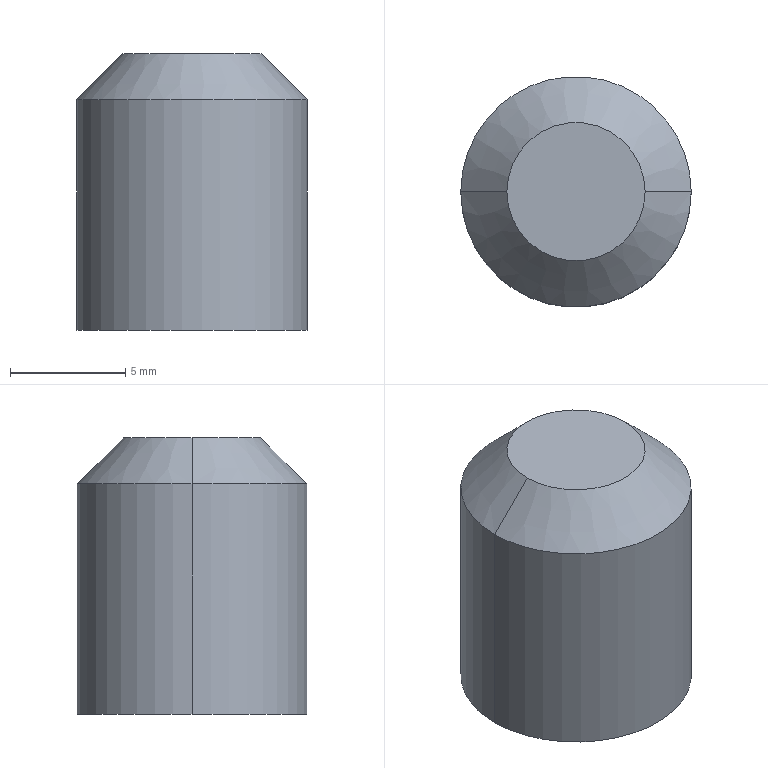Part | STEP file | ASND-0110-Body 1-26 | 1 solid | 6 faces | box 10 x 10 x 12 mm | volume 888.024 mm3 | cylinder 2 | cone 2 | plane 2 | commonest cylinder face diameters 10 x2
STEP:
#1=CARTESIAN_POINT('',(0.,0.,0.));
#2=DIRECTION('',(0.,0.,1.));
#3=DIRECTION('',(1.,0.,0.));
#4=AXIS2_PLACEMENT_3D('',#1,#2,#3);
#5=CARTESIAN_POINT('',(5.,0.,0.));
#6=VERTEX_POINT('',#5);
#7=CARTESIAN_POINT('',(-5.,0.,0.));
#8=VERTEX_POINT('',#7);
#9=CARTESIAN_POINT('',(0.,0.,0.));
#10=DIRECTION('',(0.,0.,-1.));
#11=DIRECTION('',(-1.,0.,0.));
#12=AXIS2_PLACEMENT_3D('',#9,#10,#11);
#13=CIRCLE('',#12,5.);
#14=CARTESIAN_POINT('',(0.,0.,0.));
#15=DIRECTION('',(0.,0.,1.));
#16=DIRECTION('',(-1.,0.,0.));
#17=AXIS2_PLACEMENT_3D('',#14,#15,#16);
#18=CYLINDRICAL_SURFACE('',#17,5.);
#19=CARTESIAN_POINT('',(6.283,0.));
#20=DIRECTION('',(-1.,0.));
#21=VECTOR('',#20,1.);
#22=LINE('',#19,#21);
#23=(GEOMETRIC_REPRESENTATION_CONTEXT(2)PARAMETRIC_REPRESENTATION_CONTEXT()REPRESENTATION_CONTEXT('',''));
#24=DEFINITIONAL_REPRESENTATION('',(#22),#23);
#25=PCURVE('',#18,#24);
#26=CARTESIAN_POINT('',(0.,0.,0.));
#27=DIRECTION('',(0.,0.,-1.));
#28=DIRECTION('',(0.7071,0.7071,0.));
#29=AXIS2_PLACEMENT_3D('',#26,#27,#28);
#30=PLANE('',#29);
#31=CARTESIAN_POINT('',(0.,0.));
#32=DIRECTION('',(-0.7071,-0.7071));
#33=AXIS2_PLACEMENT_2D('',#31,#32);
#34=CIRCLE('',#33,5.);
#35=(GEOMETRIC_REPRESENTATION_CONTEXT(2)PARAMETRIC_REPRESENTATION_CONTEXT()REPRESENTATION_CONTEXT('',''));
#36=DEFINITIONAL_REPRESENTATION('',(#34),#35);
#37=PCURVE('',#30,#36);
#38=SURFACE_CURVE('',#13,(#25,#37),.PCURVE_S1.);
#39=EDGE_CURVE('',#6,#8,#38,.T.);
#40=ORIENTED_EDGE('',*,*,#39,.F.);
#41=CARTESIAN_POINT('',(5.,0.,10.));
#42=VERTEX_POINT('',#41);
#43=CARTESIAN_POINT('',(5.,0.,0.));
#44=DIRECTION('',(0.,0.,1.));
#45=VECTOR('',#44,1.);
#46=LINE('',#43,#45);
#47=CARTESIAN_POINT('',(3.142,0.));
#48=DIRECTION('',(0.,1.));
#49=VECTOR('',#48,1.);
#50=LINE('',#47,#49);
#51=(GEOMETRIC_REPRESENTATION_CONTEXT(2)PARAMETRIC_REPRESENTATION_CONTEXT()REPRESENTATION_CONTEXT('',''));
#52=DEFINITIONAL_REPRESENTATION('',(#50),#51);
#53=PCURVE('',#18,#52);
#54=CARTESIAN_POINT('',(0.,0.,0.));
#55=DIRECTION('',(0.,0.,1.));
#56=DIRECTION('',(-1.,0.,0.));
#57=AXIS2_PLACEMENT_3D('',#54,#55,#56);
#58=CYLINDRICAL_SURFACE('',#57,5.);
#59=CARTESIAN_POINT('',(3.142,0.));
#60=DIRECTION('',(0.,1.));
#61=VECTOR('',#60,1.);
#62=LINE('',#59,#61);
#63=(GEOMETRIC_REPRESENTATION_CONTEXT(2)PARAMETRIC_REPRESENTATION_CONTEXT()REPRESENTATION_CONTEXT('',''));
#64=DEFINITIONAL_REPRESENTATION('',(#62),#63);
#65=PCURVE('',#58,#64);
#66=SURFACE_CURVE('',#46,(#53,#65),.PCURVE_S1.);
#67=EDGE_CURVE('',#6,#42,#66,.T.);
#68=ORIENTED_EDGE('',*,*,#67,.T.);
#69=CARTESIAN_POINT('',(-5.,0.,10.));
#70=VERTEX_POINT('',#69);
#71=CARTESIAN_POINT('',(0.,0.,10.));
#72=DIRECTION('',(0.,0.,1.));
#73=DIRECTION('',(-1.,0.,0.));
#74=AXIS2_PLACEMENT_3D('',#71,#72,#73);
#75=CIRCLE('',#74,5.);
#76=CARTESIAN_POINT('',(0.,10.));
#77=DIRECTION('',(1.,0.));
#78=VECTOR('',#77,1.);
#79=LINE('',#76,#78);
#80=(GEOMETRIC_REPRESENTATION_CONTEXT(2)PARAMETRIC_REPRESENTATION_CONTEXT()REPRESENTATION_CONTEXT('',''));
#81=DEFINITIONAL_REPRESENTATION('',(#79),#80);
#82=PCURVE('',#18,#81);
#83=CARTESIAN_POINT('',(0.,0.,11.));
#84=DIRECTION('',(0.,0.,-1.));
#85=DIRECTION('',(-1.,0.,0.));
#86=AXIS2_PLACEMENT_3D('',#83,#84,#85);
#87=CONICAL_SURFACE('',#86,4.,0.7854);
#88=CARTESIAN_POINT('',(6.283,1.));
#89=DIRECTION('',(-1.,0.));
#90=VECTOR('',#89,1.);
#91=LINE('',#88,#90);
#92=(GEOMETRIC_REPRESENTATION_CONTEXT(2)PARAMETRIC_REPRESENTATION_CONTEXT()REPRESENTATION_CONTEXT('',''));
#93=DEFINITIONAL_REPRESENTATION('',(#91),#92);
#94=PCURVE('',#87,#93);
#95=SURFACE_CURVE('',#75,(#82,#94),.PCURVE_S1.);
#96=EDGE_CURVE('',#70,#42,#95,.T.);
#97=ORIENTED_EDGE('',*,*,#96,.F.);
#98=CARTESIAN_POINT('',(-5.,0.,0.));
#99=DIRECTION('',(0.,0.,1.));
#100=VECTOR('',#99,1.);
#101=LINE('',#98,#100);
#102=CARTESIAN_POINT('',(0.,0.));
#103=DIRECTION('',(0.,1.));
#104=VECTOR('',#103,1.);
#105=LINE('',#102,#104);
#106=(GEOMETRIC_REPRESENTATION_CONTEXT(2)PARAMETRIC_REPRESENTATION_CONTEXT()REPRESENTATION_CONTEXT('',''));
#107=DEFINITIONAL_REPRESENTATION('',(#105),#106);
#108=PCURVE('',#18,#107);
#109=CARTESIAN_POINT('',(6.283,0.));
#110=DIRECTION('',(0.,1.));
#111=VECTOR('',#110,1.);
#112=LINE('',#109,#111);
#113=(GEOMETRIC_REPRESENTATION_CONTEXT(2)PARAMETRIC_REPRESENTATION_CONTEXT()REPRESENTATION_CONTEXT('',''));
#114=DEFINITIONAL_REPRESENTATION('',(#112),#113);
#115=PCURVE('',#58,#114);
#116=SURFACE_CURVE('',#101,(#108,#115),.PCURVE_S1.);
#117=EDGE_CURVE('',#8,#70,#116,.T.);
#118=ORIENTED_EDGE('',*,*,#117,.F.);
#119=EDGE_LOOP('',(#40,#68,#97,#118));
#120=FACE_BOUND('',#119,.T.);
#121=ADVANCED_FACE('',(#120),#18,.T.);
#122=CARTESIAN_POINT('',(-3.,0.,12.));
#123=VERTEX_POINT('',#122);
#124=CARTESIAN_POINT('',(3.,0.,12.));
#125=VERTEX_POINT('',#124);
#126=CARTESIAN_POINT('',(0.,0.,12.));
#127=DIRECTION('',(0.,0.,-1.));
#128=DIRECTION('',(-1.,0.,0.));
#129=AXIS2_PLACEMENT_3D('',#126,#127,#128);
#130=CIRCLE('',#129,3.);
#131=CARTESIAN_POINT('',(0.,0.,11.));
#132=DIRECTION('',(0.,0.,-1.));
#133=DIRECTION('',(-1.,0.,0.));
#134=AXIS2_PLACEMENT_3D('',#131,#132,#133);
#135=CONICAL_SURFACE('',#134,4.,0.7854);
#136=CARTESIAN_POINT('',(0.,-1.));
#137=DIRECTION('',(1.,0.));
#138=VECTOR('',#137,1.);
#139=LINE('',#136,#138);
#140=(GEOMETRIC_REPRESENTATION_CONTEXT(2)PARAMETRIC_REPRESENTATION_CONTEXT()REPRESENTATION_CONTEXT('',''));
#141=DEFINITIONAL_REPRESENTATION('',(#139),#140);
#142=PCURVE('',#135,#141);
#143=CARTESIAN_POINT('',(0.,0.,12.));
#144=DIRECTION('',(0.,0.,-1.));
#145=DIRECTION('',(0.7071,0.7071,0.));
#146=AXIS2_PLACEMENT_3D('',#143,#144,#145);
#147=PLANE('',#146);
#148=CARTESIAN_POINT('',(0.,0.));
#149=DIRECTION('',(-0.7071,-0.7071));
#150=AXIS2_PLACEMENT_2D('',#148,#149);
#151=CIRCLE('',#150,3.);
#152=(GEOMETRIC_REPRESENTATION_CONTEXT(2)PARAMETRIC_REPRESENTATION_CONTEXT()REPRESENTATION_CONTEXT('',''));
#153=DEFINITIONAL_REPRESENTATION('',(#151),#152);
#154=PCURVE('',#147,#153);
#155=SURFACE_CURVE('',#130,(#142,#154),.PCURVE_S1.);
#156=EDGE_CURVE('',#123,#125,#155,.T.);
#157=ORIENTED_EDGE('',*,*,#156,.T.);
#158=CARTESIAN_POINT('',(4.,0.,11.));
#159=DIRECTION('',(0.7071,0.,-0.7071));
#160=VECTOR('',#159,1.);
#161=LINE('',#158,#160);
#162=CARTESIAN_POINT('',(3.142,0.));
#163=DIRECTION('',(0.,1.));
#164=VECTOR('',#163,1.);
#165=LINE('',#162,#164);
#166=(GEOMETRIC_REPRESENTATION_CONTEXT(2)PARAMETRIC_REPRESENTATION_CONTEXT()REPRESENTATION_CONTEXT('',''));
#167=DEFINITIONAL_REPRESENTATION('',(#165),#166);
#168=PCURVE('',#135,#167);
#169=CARTESIAN_POINT('',(3.142,0.));
#170=DIRECTION('',(0.,1.));
#171=VECTOR('',#170,1.);
#172=LINE('',#169,#171);
#173=(GEOMETRIC_REPRESENTATION_CONTEXT(2)PARAMETRIC_REPRESENTATION_CONTEXT()REPRESENTATION_CONTEXT('',''));
#174=DEFINITIONAL_REPRESENTATION('',(#172),#173);
#175=PCURVE('',#87,#174);
#176=SURFACE_CURVE('',#161,(#168,#175),.PCURVE_S1.);
#177=EDGE_CURVE('',#125,#42,#176,.T.);
#178=ORIENTED_EDGE('',*,*,#177,.T.);
#179=CARTESIAN_POINT('',(0.,0.,10.));
#180=DIRECTION('',(0.,0.,1.));
#181=DIRECTION('',(-1.,0.,0.));
#182=AXIS2_PLACEMENT_3D('',#179,#180,#181);
#183=CIRCLE('',#182,5.);
#184=CARTESIAN_POINT('',(6.283,1.));
#185=DIRECTION('',(-1.,0.));
#186=VECTOR('',#185,1.);
#187=LINE('',#184,#186);
#188=(GEOMETRIC_REPRESENTATION_CONTEXT(2)PARAMETRIC_REPRESENTATION_CONTEXT()REPRESENTATION_CONTEXT('',''));
#189=DEFINITIONAL_REPRESENTATION('',(#187),#188);
#190=PCURVE('',#135,#189);
#191=CARTESIAN_POINT('',(0.,10.));
#192=DIRECTION('',(1.,0.));
#193=VECTOR('',#192,1.);
#194=LINE('',#191,#193);
#195=(GEOMETRIC_REPRESENTATION_CONTEXT(2)PARAMETRIC_REPRESENTATION_CONTEXT()REPRESENTATION_CONTEXT('',''));
#196=DEFINITIONAL_REPRESENTATION('',(#194),#195);
#197=PCURVE('',#58,#196);
#198=SURFACE_CURVE('',#183,(#190,#197),.PCURVE_S1.);
#199=EDGE_CURVE('',#42,#70,#198,.T.);
#200=ORIENTED_EDGE('',*,*,#199,.T.);
#201=CARTESIAN_POINT('',(-4.,0.,11.));
#202=DIRECTION('',(-0.7071,0.,-0.7071));
#203=VECTOR('',#202,1.);
#204=LINE('',#201,#203);
#205=CARTESIAN_POINT('',(0.,0.));
#206=DIRECTION('',(0.,1.));
#207=VECTOR('',#206,1.);
#208=LINE('',#205,#207);
#209=(GEOMETRIC_REPRESENTATION_CONTEXT(2)PARAMETRIC_REPRESENTATION_CONTEXT()REPRESENTATION_CONTEXT('',''));
#210=DEFINITIONAL_REPRESENTATION('',(#208),#209);
#211=PCURVE('',#135,#210);
#212=CARTESIAN_POINT('',(6.283,0.));
#213=DIRECTION('',(0.,1.));
#214=VECTOR('',#213,1.);
#215=LINE('',#212,#214);
#216=(GEOMETRIC_REPRESENTATION_CONTEXT(2)PARAMETRIC_REPRESENTATION_CONTEXT()REPRESENTATION_CONTEXT('',''));
#217=DEFINITIONAL_REPRESENTATION('',(#215),#216);
#218=PCURVE('',#87,#217);
#219=SURFACE_CURVE('',#204,(#211,#218),.PCURVE_S1.);
#220=EDGE_CURVE('',#123,#70,#219,.T.);
#221=ORIENTED_EDGE('',*,*,#220,.F.);
#222=EDGE_LOOP('',(#157,#178,#200,#221));
#223=FACE_BOUND('',#222,.T.);
#224=ADVANCED_FACE('',(#223),#135,.T.);
#225=ORIENTED_EDGE('',*,*,#177,.F.);
#226=CARTESIAN_POINT('',(0.,0.,12.));
#227=DIRECTION('',(0.,0.,-1.));
#228=DIRECTION('',(-1.,0.,0.));
#229=AXIS2_PLACEMENT_3D('',#226,#227,#228);
#230=CIRCLE('',#229,3.);
#231=CARTESIAN_POINT('',(0.,-1.));
#232=DIRECTION('',(1.,0.));
#233=VECTOR('',#232,1.);
#234=LINE('',#231,#233);
#235=(GEOMETRIC_REPRESENTATION_CONTEXT(2)PARAMETRIC_REPRESENTATION_CONTEXT()REPRESENTATION_CONTEXT('',''));
#236=DEFINITIONAL_REPRESENTATION('',(#234),#235);
#237=PCURVE('',#87,#236);
#238=CARTESIAN_POINT('',(0.,0.));
#239=DIRECTION('',(-0.7071,-0.7071));
#240=AXIS2_PLACEMENT_2D('',#238,#239);
#241=CIRCLE('',#240,3.);
#242=(GEOMETRIC_REPRESENTATION_CONTEXT(2)PARAMETRIC_REPRESENTATION_CONTEXT()REPRESENTATION_CONTEXT('',''));
#243=DEFINITIONAL_REPRESENTATION('',(#241),#242);
#244=PCURVE('',#147,#243);
#245=SURFACE_CURVE('',#230,(#237,#244),.PCURVE_S1.);
#246=EDGE_CURVE('',#125,#123,#245,.T.);
#247=ORIENTED_EDGE('',*,*,#246,.T.);
#248=ORIENTED_EDGE('',*,*,#220,.T.);
#249=ORIENTED_EDGE('',*,*,#96,.T.);
#250=EDGE_LOOP('',(#225,#247,#248,#249));
#251=FACE_BOUND('',#250,.T.);
#252=ADVANCED_FACE('',(#251),#87,.T.);
#253=ORIENTED_EDGE('',*,*,#67,.F.);
#254=CARTESIAN_POINT('',(0.,0.,0.));
#255=DIRECTION('',(0.,0.,-1.));
#256=DIRECTION('',(-1.,0.,0.));
#257=AXIS2_PLACEMENT_3D('',#254,#255,#256);
#258=CIRCLE('',#257,5.);
#259=CARTESIAN_POINT('',(6.283,0.));
#260=DIRECTION('',(-1.,0.));
#261=VECTOR('',#260,1.);
#262=LINE('',#259,#261);
#263=(GEOMETRIC_REPRESENTATION_CONTEXT(2)PARAMETRIC_REPRESENTATION_CONTEXT()REPRESENTATION_CONTEXT('',''));
#264=DEFINITIONAL_REPRESENTATION('',(#262),#263);
#265=PCURVE('',#58,#264);
#266=CARTESIAN_POINT('',(0.,0.));
#267=DIRECTION('',(-0.7071,-0.7071));
#268=AXIS2_PLACEMENT_2D('',#266,#267);
#269=CIRCLE('',#268,5.);
#270=(GEOMETRIC_REPRESENTATION_CONTEXT(2)PARAMETRIC_REPRESENTATION_CONTEXT()REPRESENTATION_CONTEXT('',''));
#271=DEFINITIONAL_REPRESENTATION('',(#269),#270);
#272=PCURVE('',#30,#271);
#273=SURFACE_CURVE('',#258,(#265,#272),.PCURVE_S1.);
#274=EDGE_CURVE('',#8,#6,#273,.T.);
#275=ORIENTED_EDGE('',*,*,#274,.F.);
#276=ORIENTED_EDGE('',*,*,#117,.T.);
#277=ORIENTED_EDGE('',*,*,#199,.F.);
#278=EDGE_LOOP('',(#253,#275,#276,#277));
#279=FACE_BOUND('',#278,.T.);
#280=ADVANCED_FACE('',(#279),#58,.T.);
#281=ORIENTED_EDGE('',*,*,#156,.F.);
#282=ORIENTED_EDGE('',*,*,#246,.F.);
#283=EDGE_LOOP('',(#281,#282));
#284=FACE_BOUND('',#283,.T.);
#285=ADVANCED_FACE('',(#284),#147,.F.);
#286=ORIENTED_EDGE('',*,*,#274,.T.);
#287=ORIENTED_EDGE('',*,*,#39,.T.);
#288=EDGE_LOOP('',(#286,#287));
#289=FACE_BOUND('',#288,.T.);
#290=ADVANCED_FACE('',(#289),#30,.T.);
#291=CLOSED_SHELL('',(#121,#224,#252,#280,#285,#290));
#292=MANIFOLD_SOLID_BREP('',#291);
#293=(LENGTH_UNIT()NAMED_UNIT(*)SI_UNIT(.MILLI.,.METRE.));
#294=UNCERTAINTY_MEASURE_WITH_UNIT(LENGTH_MEASURE(0.0000001),#293,'','');
#295=(NAMED_UNIT(*)PLANE_ANGLE_UNIT()SI_UNIT($,.RADIAN.));
#296=(NAMED_UNIT(*)SI_UNIT($,.STERADIAN.)SOLID_ANGLE_UNIT());
#297=(GEOMETRIC_REPRESENTATION_CONTEXT(3)GLOBAL_UNCERTAINTY_ASSIGNED_CONTEXT((#294))GLOBAL_UNIT_ASSIGNED_CONTEXT((#293,#295,#296))REPRESENTATION_CONTEXT('',''));
#298=ADVANCED_BREP_SHAPE_REPRESENTATION('',(#4,#292),#297);